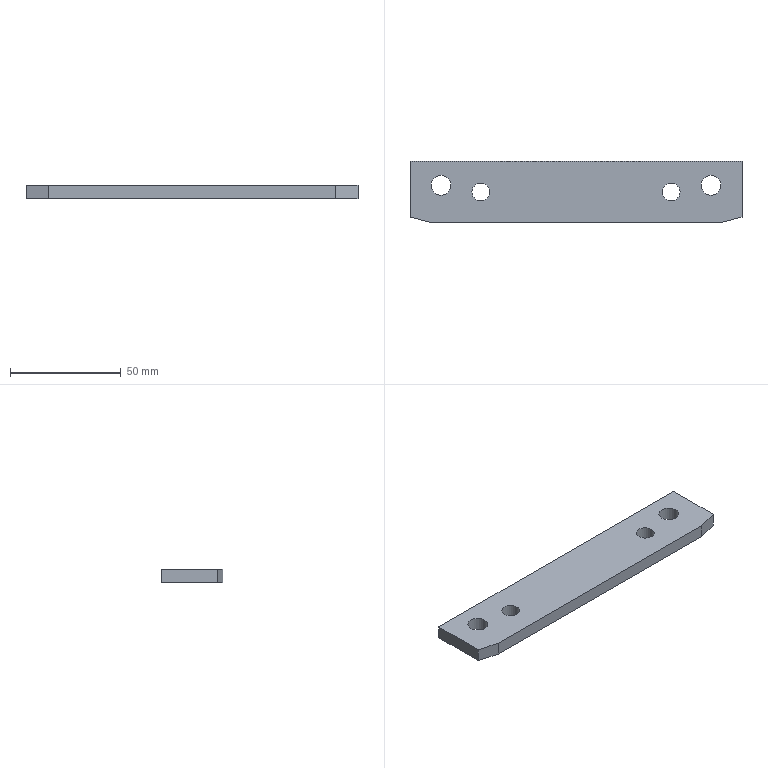Part | STEP file | gslz 2016.10.28-13_id1578_x_t | 1 solid | 12 faces | box 150 x 28 x 6 mm | volume 23673 mm3 | plane 8 | cylinder 4 | commonest cylinder face diameters 8 x2 9 x2
STEP:
#1=CARTESIAN_POINT('',(0.,0.,0.));
#2=DIRECTION('',(0.,0.,1.));
#3=DIRECTION('',(1.,0.,0.));
#4=AXIS2_PLACEMENT_3D('',#1,#2,#3);
#5=CARTESIAN_POINT('',(-1584.002,284.2,6.));
#6=VERTEX_POINT('',#5);
#7=CARTESIAN_POINT('',(-1592.002,284.2,6.));
#8=VERTEX_POINT('',#7);
#9=CARTESIAN_POINT('',(-1588.002,284.2,6.));
#10=DIRECTION('',(0.,0.,1.));
#11=DIRECTION('',(-1.,0.,0.));
#12=AXIS2_PLACEMENT_3D('',#9,#10,#11);
#13=CIRCLE('',#12,4.);
#14=CARTESIAN_POINT('',(-1588.002,284.2,-73.));
#15=DIRECTION('',(0.,0.,1.));
#16=DIRECTION('',(1.,0.,0.));
#17=AXIS2_PLACEMENT_3D('',#14,#15,#16);
#18=CYLINDRICAL_SURFACE('',#17,4.);
#19=CARTESIAN_POINT('',(-3.142,79.));
#20=DIRECTION('',(1.,0.));
#21=VECTOR('',#20,1.);
#22=LINE('',#19,#21);
#23=(GEOMETRIC_REPRESENTATION_CONTEXT(2)PARAMETRIC_REPRESENTATION_CONTEXT()REPRESENTATION_CONTEXT('',''));
#24=DEFINITIONAL_REPRESENTATION('',(#22),#23);
#25=PCURVE('',#18,#24);
#26=CARTESIAN_POINT('',(-1585.002,267.7,6.));
#27=DIRECTION('',(0.,0.,-1.));
#28=DIRECTION('',(-1.,0.,0.));
#29=AXIS2_PLACEMENT_3D('',#26,#27,#28);
#30=PLANE('',#29);
#31=CARTESIAN_POINT('',(7.,16.5));
#32=CARTESIAN_POINT('',(7.,9.572));
#33=CARTESIAN_POINT('',(1.,13.036));
#34=CARTESIAN_POINT('',(-5.,16.5));
#35=CARTESIAN_POINT('',(1.,19.964));
#36=CARTESIAN_POINT('',(7.,23.428));
#37=CARTESIAN_POINT('',(7.,16.5));
#38=(BOUNDED_CURVE()B_SPLINE_CURVE(2,(#31,#32,#33,#34,#35,#36,#37),.UNSPECIFIED.,.T.,.F.)B_SPLINE_CURVE_WITH_KNOTS((1,2,2,2,2,1),(-2.094,0.,2.094,4.189,6.283,8.378),.UNSPECIFIED.)CURVE()GEOMETRIC_REPRESENTATION_ITEM()RATIONAL_B_SPLINE_CURVE((1.,0.5,1.,0.5,1.,0.5,1.))REPRESENTATION_ITEM(''));
#39=(GEOMETRIC_REPRESENTATION_CONTEXT(2)PARAMETRIC_REPRESENTATION_CONTEXT()REPRESENTATION_CONTEXT('',''));
#40=DEFINITIONAL_REPRESENTATION('',(#38),#39);
#41=PCURVE('',#30,#40);
#42=SURFACE_CURVE('',#13,(#25,#41),.PCURVE_S1.);
#43=EDGE_CURVE('',#6,#8,#42,.T.);
#44=ORIENTED_EDGE('',*,*,#43,.F.);
#45=CARTESIAN_POINT('',(-1584.002,284.2,0.));
#46=VERTEX_POINT('',#45);
#47=CARTESIAN_POINT('',(-1584.002,284.2,0.));
#48=CARTESIAN_POINT('',(-1584.002,284.2,6.));
#49=B_SPLINE_CURVE_WITH_KNOTS('',1,(#47,#48),.UNSPECIFIED.,.F.,.F.,(2,2),(73.,79.),.PIECEWISE_BEZIER_KNOTS.);
#50=CARTESIAN_POINT('',(0.,0.));
#51=DIRECTION('',(0.,1.));
#52=VECTOR('',#51,1.);
#53=LINE('',#50,#52);
#54=(GEOMETRIC_REPRESENTATION_CONTEXT(2)PARAMETRIC_REPRESENTATION_CONTEXT()REPRESENTATION_CONTEXT('',''));
#55=DEFINITIONAL_REPRESENTATION('',(#53),#54);
#56=PCURVE('',#18,#55);
#57=CARTESIAN_POINT('',(6.283,0.));
#58=DIRECTION('',(0.,1.));
#59=VECTOR('',#58,1.);
#60=LINE('',#57,#59);
#61=(GEOMETRIC_REPRESENTATION_CONTEXT(2)PARAMETRIC_REPRESENTATION_CONTEXT()REPRESENTATION_CONTEXT('',''));
#62=DEFINITIONAL_REPRESENTATION('',(#60),#61);
#63=PCURVE('',#18,#62);
#64=SEAM_CURVE('',#49,(#56,#63),.PCURVE_S1.);
#65=EDGE_CURVE('',#46,#6,#64,.T.);
#66=ORIENTED_EDGE('',*,*,#65,.F.);
#67=CARTESIAN_POINT('',(-1588.002,284.2,0.));
#68=DIRECTION('',(0.,0.,-1.));
#69=DIRECTION('',(1.,0.,0.));
#70=AXIS2_PLACEMENT_3D('',#67,#68,#69);
#71=CIRCLE('',#70,4.);
#72=CARTESIAN_POINT('',(6.283,73.));
#73=DIRECTION('',(-1.,0.));
#74=VECTOR('',#73,1.);
#75=LINE('',#72,#74);
#76=(GEOMETRIC_REPRESENTATION_CONTEXT(2)PARAMETRIC_REPRESENTATION_CONTEXT()REPRESENTATION_CONTEXT('',''));
#77=DEFINITIONAL_REPRESENTATION('',(#75),#76);
#78=PCURVE('',#18,#77);
#79=CARTESIAN_POINT('',(-1625.002,298.2,0.));
#80=DIRECTION('',(0.,0.,1.));
#81=DIRECTION('',(1.,0.,0.));
#82=AXIS2_PLACEMENT_3D('',#79,#80,#81);
#83=PLANE('',#82);
#84=CARTESIAN_POINT('',(41.,-14.));
#85=CARTESIAN_POINT('',(41.,-20.928));
#86=CARTESIAN_POINT('',(35.,-17.464));
#87=CARTESIAN_POINT('',(29.,-14.));
#88=CARTESIAN_POINT('',(35.,-10.536));
#89=CARTESIAN_POINT('',(41.,-7.072));
#90=CARTESIAN_POINT('',(41.,-14.));
#91=(BOUNDED_CURVE()B_SPLINE_CURVE(2,(#84,#85,#86,#87,#88,#89,#90),.UNSPECIFIED.,.T.,.F.)B_SPLINE_CURVE_WITH_KNOTS((1,2,2,2,2,1),(-2.094,0.,2.094,4.189,6.283,8.378),.UNSPECIFIED.)CURVE()GEOMETRIC_REPRESENTATION_ITEM()RATIONAL_B_SPLINE_CURVE((1.,0.5,1.,0.5,1.,0.5,1.))REPRESENTATION_ITEM(''));
#92=(GEOMETRIC_REPRESENTATION_CONTEXT(2)PARAMETRIC_REPRESENTATION_CONTEXT()REPRESENTATION_CONTEXT('',''));
#93=DEFINITIONAL_REPRESENTATION('',(#91),#92);
#94=PCURVE('',#83,#93);
#95=SURFACE_CURVE('',#71,(#78,#94),.PCURVE_S1.);
#96=EDGE_CURVE('',#46,#46,#95,.T.);
#97=ORIENTED_EDGE('',*,*,#96,.F.);
#98=ORIENTED_EDGE('',*,*,#65,.T.);
#99=CARTESIAN_POINT('',(-1588.002,284.2,6.));
#100=DIRECTION('',(0.,0.,1.));
#101=DIRECTION('',(-1.,0.,0.));
#102=AXIS2_PLACEMENT_3D('',#99,#100,#101);
#103=CIRCLE('',#102,4.);
#104=CARTESIAN_POINT('',(3.142,79.));
#105=DIRECTION('',(1.,0.));
#106=VECTOR('',#105,1.);
#107=LINE('',#104,#106);
#108=(GEOMETRIC_REPRESENTATION_CONTEXT(2)PARAMETRIC_REPRESENTATION_CONTEXT()REPRESENTATION_CONTEXT('',''));
#109=DEFINITIONAL_REPRESENTATION('',(#107),#108);
#110=PCURVE('',#18,#109);
#111=CARTESIAN_POINT('',(7.,16.5));
#112=CARTESIAN_POINT('',(7.,9.572));
#113=CARTESIAN_POINT('',(1.,13.036));
#114=CARTESIAN_POINT('',(-5.,16.5));
#115=CARTESIAN_POINT('',(1.,19.964));
#116=CARTESIAN_POINT('',(7.,23.428));
#117=CARTESIAN_POINT('',(7.,16.5));
#118=(BOUNDED_CURVE()B_SPLINE_CURVE(2,(#111,#112,#113,#114,#115,#116,#117),.UNSPECIFIED.,.T.,.F.)B_SPLINE_CURVE_WITH_KNOTS((1,2,2,2,2,1),(-2.094,0.,2.094,4.189,6.283,8.378),.UNSPECIFIED.)CURVE()GEOMETRIC_REPRESENTATION_ITEM()RATIONAL_B_SPLINE_CURVE((1.,0.5,1.,0.5,1.,0.5,1.))REPRESENTATION_ITEM(''));
#119=(GEOMETRIC_REPRESENTATION_CONTEXT(2)PARAMETRIC_REPRESENTATION_CONTEXT()REPRESENTATION_CONTEXT('',''));
#120=DEFINITIONAL_REPRESENTATION('',(#118),#119);
#121=PCURVE('',#30,#120);
#122=SURFACE_CURVE('',#103,(#110,#121),.PCURVE_S1.);
#123=EDGE_CURVE('',#8,#6,#122,.T.);
#124=ORIENTED_EDGE('',*,*,#123,.F.);
#125=EDGE_LOOP('',(#44,#66,#97,#98,#124));
#126=FACE_BOUND('',#125,.F.);
#127=ADVANCED_FACE('',(#126),#18,.F.);
#128=CARTESIAN_POINT('',(-1506.002,284.2,6.));
#129=VERTEX_POINT('',#128);
#130=CARTESIAN_POINT('',(-1498.002,284.2,6.));
#131=VERTEX_POINT('',#130);
#132=CARTESIAN_POINT('',(-1502.002,284.2,6.));
#133=DIRECTION('',(0.,0.,-1.));
#134=DIRECTION('',(-1.,0.,0.));
#135=AXIS2_PLACEMENT_3D('',#132,#133,#134);
#136=CIRCLE('',#135,4.);
#137=CARTESIAN_POINT('',(-1502.002,284.2,-73.));
#138=DIRECTION('',(0.,0.,1.));
#139=DIRECTION('',(1.,0.,0.));
#140=AXIS2_PLACEMENT_3D('',#137,#138,#139);
#141=CYLINDRICAL_SURFACE('',#140,4.);
#142=CARTESIAN_POINT('',(3.142,79.));
#143=DIRECTION('',(-1.,0.));
#144=VECTOR('',#143,1.);
#145=LINE('',#142,#144);
#146=(GEOMETRIC_REPRESENTATION_CONTEXT(2)PARAMETRIC_REPRESENTATION_CONTEXT()REPRESENTATION_CONTEXT('',''));
#147=DEFINITIONAL_REPRESENTATION('',(#145),#146);
#148=PCURVE('',#141,#147);
#149=CARTESIAN_POINT('',(-83.,16.5));
#150=DIRECTION('',(1.,0.));
#151=AXIS2_PLACEMENT_2D('',#149,#150);
#152=CIRCLE('',#151,4.);
#153=(GEOMETRIC_REPRESENTATION_CONTEXT(2)PARAMETRIC_REPRESENTATION_CONTEXT()REPRESENTATION_CONTEXT('',''));
#154=DEFINITIONAL_REPRESENTATION('',(#152),#153);
#155=PCURVE('',#30,#154);
#156=SURFACE_CURVE('',#136,(#148,#155),.PCURVE_S1.);
#157=EDGE_CURVE('',#129,#131,#156,.T.);
#158=ORIENTED_EDGE('',*,*,#157,.T.);
#159=CARTESIAN_POINT('',(-1498.002,284.2,0.));
#160=VERTEX_POINT('',#159);
#161=CARTESIAN_POINT('',(-1498.002,284.2,0.));
#162=CARTESIAN_POINT('',(-1498.002,284.2,6.));
#163=B_SPLINE_CURVE_WITH_KNOTS('',1,(#161,#162),.UNSPECIFIED.,.F.,.F.,(2,2),(73.,79.),.PIECEWISE_BEZIER_KNOTS.);
#164=CARTESIAN_POINT('',(0.,0.));
#165=DIRECTION('',(0.,1.));
#166=VECTOR('',#165,1.);
#167=LINE('',#164,#166);
#168=(GEOMETRIC_REPRESENTATION_CONTEXT(2)PARAMETRIC_REPRESENTATION_CONTEXT()REPRESENTATION_CONTEXT('',''));
#169=DEFINITIONAL_REPRESENTATION('',(#167),#168);
#170=PCURVE('',#141,#169);
#171=CARTESIAN_POINT('',(6.283,0.));
#172=DIRECTION('',(0.,1.));
#173=VECTOR('',#172,1.);
#174=LINE('',#171,#173);
#175=(GEOMETRIC_REPRESENTATION_CONTEXT(2)PARAMETRIC_REPRESENTATION_CONTEXT()REPRESENTATION_CONTEXT('',''));
#176=DEFINITIONAL_REPRESENTATION('',(#174),#175);
#177=PCURVE('',#141,#176);
#178=SEAM_CURVE('',#163,(#170,#177),.PCURVE_S1.);
#179=EDGE_CURVE('',#160,#131,#178,.T.);
#180=ORIENTED_EDGE('',*,*,#179,.F.);
#181=CARTESIAN_POINT('',(-1502.002,284.2,0.));
#182=DIRECTION('',(0.,0.,1.));
#183=DIRECTION('',(1.,0.,0.));
#184=AXIS2_PLACEMENT_3D('',#181,#182,#183);
#185=CIRCLE('',#184,4.);
#186=CARTESIAN_POINT('',(0.,73.));
#187=DIRECTION('',(1.,0.));
#188=VECTOR('',#187,1.);
#189=LINE('',#186,#188);
#190=(GEOMETRIC_REPRESENTATION_CONTEXT(2)PARAMETRIC_REPRESENTATION_CONTEXT()REPRESENTATION_CONTEXT('',''));
#191=DEFINITIONAL_REPRESENTATION('',(#189),#190);
#192=PCURVE('',#141,#191);
#193=CARTESIAN_POINT('',(123.,-14.));
#194=DIRECTION('',(1.,0.));
#195=AXIS2_PLACEMENT_2D('',#193,#194);
#196=CIRCLE('',#195,4.);
#197=(GEOMETRIC_REPRESENTATION_CONTEXT(2)PARAMETRIC_REPRESENTATION_CONTEXT()REPRESENTATION_CONTEXT('',''));
#198=DEFINITIONAL_REPRESENTATION('',(#196),#197);
#199=PCURVE('',#83,#198);
#200=SURFACE_CURVE('',#185,(#192,#199),.PCURVE_S1.);
#201=EDGE_CURVE('',#160,#160,#200,.T.);
#202=ORIENTED_EDGE('',*,*,#201,.T.);
#203=ORIENTED_EDGE('',*,*,#179,.T.);
#204=CARTESIAN_POINT('',(-1502.002,284.2,6.));
#205=DIRECTION('',(0.,0.,-1.));
#206=DIRECTION('',(-1.,0.,0.));
#207=AXIS2_PLACEMENT_3D('',#204,#205,#206);
#208=CIRCLE('',#207,4.);
#209=CARTESIAN_POINT('',(9.425,79.));
#210=DIRECTION('',(-1.,0.));
#211=VECTOR('',#210,1.);
#212=LINE('',#209,#211);
#213=(GEOMETRIC_REPRESENTATION_CONTEXT(2)PARAMETRIC_REPRESENTATION_CONTEXT()REPRESENTATION_CONTEXT('',''));
#214=DEFINITIONAL_REPRESENTATION('',(#212),#213);
#215=PCURVE('',#141,#214);
#216=CARTESIAN_POINT('',(-83.,16.5));
#217=DIRECTION('',(1.,0.));
#218=AXIS2_PLACEMENT_2D('',#216,#217);
#219=CIRCLE('',#218,4.);
#220=(GEOMETRIC_REPRESENTATION_CONTEXT(2)PARAMETRIC_REPRESENTATION_CONTEXT()REPRESENTATION_CONTEXT('',''));
#221=DEFINITIONAL_REPRESENTATION('',(#219),#220);
#222=PCURVE('',#30,#221);
#223=SURFACE_CURVE('',#208,(#215,#222),.PCURVE_S1.);
#224=EDGE_CURVE('',#131,#129,#223,.T.);
#225=ORIENTED_EDGE('',*,*,#224,.T.);
#226=EDGE_LOOP('',(#158,#180,#202,#203,#225));
#227=FACE_BOUND('',#226,.F.);
#228=ADVANCED_FACE('',(#227),#141,.F.);
#229=CARTESIAN_POINT('',(-1610.502,287.2,6.));
#230=VERTEX_POINT('',#229);
#231=CARTESIAN_POINT('',(-1606.002,287.2,6.));
#232=DIRECTION('',(0.,0.,-1.));
#233=DIRECTION('',(-1.,0.,0.));
#234=AXIS2_PLACEMENT_3D('',#231,#232,#233);
#235=CIRCLE('',#234,4.5);
#236=CARTESIAN_POINT('',(-1606.002,287.2,47.));
#237=DIRECTION('',(0.,0.,-1.));
#238=DIRECTION('',(-1.,0.,0.));
#239=AXIS2_PLACEMENT_3D('',#236,#237,#238);
#240=CYLINDRICAL_SURFACE('',#239,4.5);
#241=CARTESIAN_POINT('',(0.,41.));
#242=DIRECTION('',(1.,0.));
#243=VECTOR('',#242,1.);
#244=LINE('',#241,#243);
#245=(GEOMETRIC_REPRESENTATION_CONTEXT(2)PARAMETRIC_REPRESENTATION_CONTEXT()REPRESENTATION_CONTEXT('',''));
#246=DEFINITIONAL_REPRESENTATION('',(#244),#245);
#247=PCURVE('',#240,#246);
#248=CARTESIAN_POINT('',(21.,19.5));
#249=DIRECTION('',(1.,0.));
#250=AXIS2_PLACEMENT_2D('',#248,#249);
#251=CIRCLE('',#250,4.5);
#252=(GEOMETRIC_REPRESENTATION_CONTEXT(2)PARAMETRIC_REPRESENTATION_CONTEXT()REPRESENTATION_CONTEXT('',''));
#253=DEFINITIONAL_REPRESENTATION('',(#251),#252);
#254=PCURVE('',#30,#253);
#255=SURFACE_CURVE('',#235,(#247,#254),.PCURVE_S1.);
#256=EDGE_CURVE('',#230,#230,#255,.T.);
#257=ORIENTED_EDGE('',*,*,#256,.T.);
#258=CARTESIAN_POINT('',(-1610.502,287.2,0.));
#259=VERTEX_POINT('',#258);
#260=CARTESIAN_POINT('',(-1610.502,287.2,6.));
#261=CARTESIAN_POINT('',(-1610.502,287.2,0.));
#262=B_SPLINE_CURVE_WITH_KNOTS('',1,(#260,#261),.UNSPECIFIED.,.F.,.F.,(2,2),(41.,47.),.PIECEWISE_BEZIER_KNOTS.);
#263=CARTESIAN_POINT('',(6.283,0.));
#264=DIRECTION('',(0.,1.));
#265=VECTOR('',#264,1.);
#266=LINE('',#263,#265);
#267=(GEOMETRIC_REPRESENTATION_CONTEXT(2)PARAMETRIC_REPRESENTATION_CONTEXT()REPRESENTATION_CONTEXT('',''));
#268=DEFINITIONAL_REPRESENTATION('',(#266),#267);
#269=PCURVE('',#240,#268);
#270=CARTESIAN_POINT('',(0.,0.));
#271=DIRECTION('',(0.,1.));
#272=VECTOR('',#271,1.);
#273=LINE('',#270,#272);
#274=(GEOMETRIC_REPRESENTATION_CONTEXT(2)PARAMETRIC_REPRESENTATION_CONTEXT()REPRESENTATION_CONTEXT('',''));
#275=DEFINITIONAL_REPRESENTATION('',(#273),#274);
#276=PCURVE('',#240,#275);
#277=SEAM_CURVE('',#262,(#269,#276),.PCURVE_S1.);
#278=EDGE_CURVE('',#230,#259,#277,.T.);
#279=ORIENTED_EDGE('',*,*,#278,.T.);
#280=CARTESIAN_POINT('',(-1601.502,287.2,0.));
#281=VERTEX_POINT('',#280);
#282=CARTESIAN_POINT('',(-1606.002,287.2,0.));
#283=DIRECTION('',(0.,0.,1.));
#284=DIRECTION('',(1.,0.,0.));
#285=AXIS2_PLACEMENT_3D('',#282,#283,#284);
#286=CIRCLE('',#285,4.5);
#287=CARTESIAN_POINT('',(9.425,47.));
#288=DIRECTION('',(-1.,0.));
#289=VECTOR('',#288,1.);
#290=LINE('',#287,#289);
#291=(GEOMETRIC_REPRESENTATION_CONTEXT(2)PARAMETRIC_REPRESENTATION_CONTEXT()REPRESENTATION_CONTEXT('',''));
#292=DEFINITIONAL_REPRESENTATION('',(#290),#291);
#293=PCURVE('',#240,#292);
#294=CARTESIAN_POINT('',(19.,-11.));
#295=DIRECTION('',(1.,0.));
#296=AXIS2_PLACEMENT_2D('',#294,#295);
#297=CIRCLE('',#296,4.5);
#298=(GEOMETRIC_REPRESENTATION_CONTEXT(2)PARAMETRIC_REPRESENTATION_CONTEXT()REPRESENTATION_CONTEXT('',''));
#299=DEFINITIONAL_REPRESENTATION('',(#297),#298);
#300=PCURVE('',#83,#299);
#301=SURFACE_CURVE('',#286,(#293,#300),.PCURVE_S1.);
#302=EDGE_CURVE('',#259,#281,#301,.T.);
#303=ORIENTED_EDGE('',*,*,#302,.T.);
#304=CARTESIAN_POINT('',(-1606.002,287.2,0.));
#305=DIRECTION('',(0.,0.,1.));
#306=DIRECTION('',(1.,0.,0.));
#307=AXIS2_PLACEMENT_3D('',#304,#305,#306);
#308=CIRCLE('',#307,4.5);
#309=CARTESIAN_POINT('',(3.142,47.));
#310=DIRECTION('',(-1.,0.));
#311=VECTOR('',#310,1.);
#312=LINE('',#309,#311);
#313=(GEOMETRIC_REPRESENTATION_CONTEXT(2)PARAMETRIC_REPRESENTATION_CONTEXT()REPRESENTATION_CONTEXT('',''));
#314=DEFINITIONAL_REPRESENTATION('',(#312),#313);
#315=PCURVE('',#240,#314);
#316=CARTESIAN_POINT('',(19.,-11.));
#317=DIRECTION('',(1.,0.));
#318=AXIS2_PLACEMENT_2D('',#316,#317);
#319=CIRCLE('',#318,4.5);
#320=(GEOMETRIC_REPRESENTATION_CONTEXT(2)PARAMETRIC_REPRESENTATION_CONTEXT()REPRESENTATION_CONTEXT('',''));
#321=DEFINITIONAL_REPRESENTATION('',(#319),#320);
#322=PCURVE('',#83,#321);
#323=SURFACE_CURVE('',#308,(#315,#322),.PCURVE_S1.);
#324=EDGE_CURVE('',#281,#259,#323,.T.);
#325=ORIENTED_EDGE('',*,*,#324,.T.);
#326=ORIENTED_EDGE('',*,*,#278,.F.);
#327=EDGE_LOOP('',(#257,#279,#303,#325,#326));
#328=FACE_BOUND('',#327,.F.);
#329=ADVANCED_FACE('',(#328),#240,.F.);
#330=CARTESIAN_POINT('',(-1480.001,270.2,0.));
#331=VERTEX_POINT('',#330);
#332=CARTESIAN_POINT('',(-1480.001,270.2,6.));
#333=VERTEX_POINT('',#332);
#334=CARTESIAN_POINT('',(-1480.001,270.2,8.));
#335=DIRECTION('',(0.,0.,1.));
#336=VECTOR('',#335,1.);
#337=LINE('',#334,#336);
#338=CARTESIAN_POINT('',(-1615.,270.2,8.));
#339=DIRECTION('',(0.,1.,0.));
#340=DIRECTION('',(0.,0.,1.));
#341=AXIS2_PLACEMENT_3D('',#338,#339,#340);
#342=PLANE('',#341);
#343=CARTESIAN_POINT('',(0.,134.999));
#344=DIRECTION('',(1.,0.));
#345=VECTOR('',#344,1.);
#346=LINE('',#343,#345);
#347=(GEOMETRIC_REPRESENTATION_CONTEXT(2)PARAMETRIC_REPRESENTATION_CONTEXT()REPRESENTATION_CONTEXT('',''));
#348=DEFINITIONAL_REPRESENTATION('',(#346),#347);
#349=PCURVE('',#342,#348);
#350=CARTESIAN_POINT('',(-1480.001,270.2,8.));
#351=DIRECTION('',(-0.2588,0.9659,0.));
#352=DIRECTION('',(-0.9659,-0.2588,0.));
#353=AXIS2_PLACEMENT_3D('',#350,#351,#352);
#354=PLANE('',#353);
#355=CARTESIAN_POINT('',(0.,0.));
#356=DIRECTION('',(0.,1.));
#357=VECTOR('',#356,1.);
#358=LINE('',#355,#357);
#359=(GEOMETRIC_REPRESENTATION_CONTEXT(2)PARAMETRIC_REPRESENTATION_CONTEXT()REPRESENTATION_CONTEXT('',''));
#360=DEFINITIONAL_REPRESENTATION('',(#358),#359);
#361=PCURVE('',#354,#360);
#362=SURFACE_CURVE('',#337,(#349,#361),.PCURVE_S1.);
#363=EDGE_CURVE('',#331,#333,#362,.T.);
#364=ORIENTED_EDGE('',*,*,#363,.T.);
#365=CARTESIAN_POINT('',(-1610.,270.2,6.));
#366=VERTEX_POINT('',#365);
#367=CARTESIAN_POINT('',(-1615.,270.2,6.));
#368=DIRECTION('',(-1.,0.,0.));
#369=VECTOR('',#368,1.);
#370=LINE('',#367,#369);
#371=CARTESIAN_POINT('',(-2.,0.));
#372=DIRECTION('',(0.,-1.));
#373=VECTOR('',#372,1.);
#374=LINE('',#371,#373);
#375=(GEOMETRIC_REPRESENTATION_CONTEXT(2)PARAMETRIC_REPRESENTATION_CONTEXT()REPRESENTATION_CONTEXT('',''));
#376=DEFINITIONAL_REPRESENTATION('',(#374),#375);
#377=PCURVE('',#342,#376);
#378=CARTESIAN_POINT('',(29.998,2.5));
#379=DIRECTION('',(1.,0.));
#380=VECTOR('',#379,1.);
#381=LINE('',#378,#380);
#382=(GEOMETRIC_REPRESENTATION_CONTEXT(2)PARAMETRIC_REPRESENTATION_CONTEXT()REPRESENTATION_CONTEXT('',''));
#383=DEFINITIONAL_REPRESENTATION('',(#381),#382);
#384=PCURVE('',#30,#383);
#385=SURFACE_CURVE('',#370,(#377,#384),.PCURVE_S1.);
#386=EDGE_CURVE('',#333,#366,#385,.T.);
#387=ORIENTED_EDGE('',*,*,#386,.T.);
#388=CARTESIAN_POINT('',(-1610.,270.2,0.));
#389=VERTEX_POINT('',#388);
#390=CARTESIAN_POINT('',(-1610.,270.2,8.));
#391=DIRECTION('',(0.,0.,1.));
#392=VECTOR('',#391,1.);
#393=LINE('',#390,#392);
#394=CARTESIAN_POINT('',(0.,5.));
#395=DIRECTION('',(1.,0.));
#396=VECTOR('',#395,1.);
#397=LINE('',#394,#396);
#398=(GEOMETRIC_REPRESENTATION_CONTEXT(2)PARAMETRIC_REPRESENTATION_CONTEXT()REPRESENTATION_CONTEXT('',''));
#399=DEFINITIONAL_REPRESENTATION('',(#397),#398);
#400=PCURVE('',#342,#399);
#401=CARTESIAN_POINT('',(-1620.002,272.88,8.));
#402=DIRECTION('',(0.2588,0.9659,0.));
#403=DIRECTION('',(-0.9659,0.2588,0.));
#404=AXIS2_PLACEMENT_3D('',#401,#402,#403);
#405=PLANE('',#404);
#406=CARTESIAN_POINT('',(-10.355,0.));
#407=DIRECTION('',(0.,1.));
#408=VECTOR('',#407,1.);
#409=LINE('',#406,#408);
#410=(GEOMETRIC_REPRESENTATION_CONTEXT(2)PARAMETRIC_REPRESENTATION_CONTEXT()REPRESENTATION_CONTEXT('',''));
#411=DEFINITIONAL_REPRESENTATION('',(#409),#410);
#412=PCURVE('',#405,#411);
#413=SURFACE_CURVE('',#393,(#400,#412),.PCURVE_S1.);
#414=EDGE_CURVE('',#389,#366,#413,.T.);
#415=ORIENTED_EDGE('',*,*,#414,.F.);
#416=CARTESIAN_POINT('',(-1615.,270.2,0.));
#417=DIRECTION('',(1.,0.,0.));
#418=VECTOR('',#417,1.);
#419=LINE('',#416,#418);
#420=CARTESIAN_POINT('',(-8.,0.));
#421=DIRECTION('',(0.,1.));
#422=VECTOR('',#421,1.);
#423=LINE('',#420,#422);
#424=(GEOMETRIC_REPRESENTATION_CONTEXT(2)PARAMETRIC_REPRESENTATION_CONTEXT()REPRESENTATION_CONTEXT('',''));
#425=DEFINITIONAL_REPRESENTATION('',(#423),#424);
#426=PCURVE('',#342,#425);
#427=CARTESIAN_POINT('',(10.002,-28.));
#428=DIRECTION('',(1.,0.));
#429=VECTOR('',#428,1.);
#430=LINE('',#427,#429);
#431=(GEOMETRIC_REPRESENTATION_CONTEXT(2)PARAMETRIC_REPRESENTATION_CONTEXT()REPRESENTATION_CONTEXT('',''));
#432=DEFINITIONAL_REPRESENTATION('',(#430),#431);
#433=PCURVE('',#83,#432);
#434=SURFACE_CURVE('',#419,(#426,#433),.PCURVE_S1.);
#435=EDGE_CURVE('',#389,#331,#434,.T.);
#436=ORIENTED_EDGE('',*,*,#435,.T.);
#437=EDGE_LOOP('',(#364,#387,#415,#436));
#438=FACE_BOUND('',#437,.T.);
#439=ADVANCED_FACE('',(#438),#342,.F.);
#440=CARTESIAN_POINT('',(-1470.002,272.879,6.));
#441=VERTEX_POINT('',#440);
#442=CARTESIAN_POINT('',(-1470.002,272.879,0.));
#443=VERTEX_POINT('',#442);
#444=CARTESIAN_POINT('',(-1470.002,272.879,8.));
#445=DIRECTION('',(0.,0.,-1.));
#446=VECTOR('',#445,1.);
#447=LINE('',#444,#446);
#448=CARTESIAN_POINT('',(-10.352,0.));
#449=DIRECTION('',(0.,-1.));
#450=VECTOR('',#449,1.);
#451=LINE('',#448,#450);
#452=(GEOMETRIC_REPRESENTATION_CONTEXT(2)PARAMETRIC_REPRESENTATION_CONTEXT()REPRESENTATION_CONTEXT('',''));
#453=DEFINITIONAL_REPRESENTATION('',(#451),#452);
#454=PCURVE('',#354,#453);
#455=CARTESIAN_POINT('',(-1470.002,265.2,16.));
#456=DIRECTION('',(-1.,0.,0.));
#457=DIRECTION('',(0.,0.,1.));
#458=AXIS2_PLACEMENT_3D('',#455,#456,#457);
#459=PLANE('',#458);
#460=CARTESIAN_POINT('',(-8.,7.679));
#461=DIRECTION('',(-1.,0.));
#462=VECTOR('',#461,1.);
#463=LINE('',#460,#462);
#464=(GEOMETRIC_REPRESENTATION_CONTEXT(2)PARAMETRIC_REPRESENTATION_CONTEXT()REPRESENTATION_CONTEXT('',''));
#465=DEFINITIONAL_REPRESENTATION('',(#463),#464);
#466=PCURVE('',#459,#465);
#467=SURFACE_CURVE('',#447,(#454,#466),.PCURVE_S1.);
#468=EDGE_CURVE('',#441,#443,#467,.T.);
#469=ORIENTED_EDGE('',*,*,#468,.F.);
#470=CARTESIAN_POINT('',(-1480.001,270.2,6.));
#471=DIRECTION('',(-0.9659,-0.2588,0.));
#472=VECTOR('',#471,1.);
#473=LINE('',#470,#472);
#474=CARTESIAN_POINT('',(0.,-2.));
#475=DIRECTION('',(1.,0.));
#476=VECTOR('',#475,1.);
#477=LINE('',#474,#476);
#478=(GEOMETRIC_REPRESENTATION_CONTEXT(2)PARAMETRIC_REPRESENTATION_CONTEXT()REPRESENTATION_CONTEXT('',''));
#479=DEFINITIONAL_REPRESENTATION('',(#477),#478);
#480=PCURVE('',#354,#479);
#481=CARTESIAN_POINT('',(-105.001,2.5));
#482=DIRECTION('',(0.9659,-0.2588));
#483=VECTOR('',#482,1.);
#484=LINE('',#481,#483);
#485=(GEOMETRIC_REPRESENTATION_CONTEXT(2)PARAMETRIC_REPRESENTATION_CONTEXT()REPRESENTATION_CONTEXT('',''));
#486=DEFINITIONAL_REPRESENTATION('',(#484),#485);
#487=PCURVE('',#30,#486);
#488=SURFACE_CURVE('',#473,(#480,#487),.PCURVE_S1.);
#489=EDGE_CURVE('',#441,#333,#488,.T.);
#490=ORIENTED_EDGE('',*,*,#489,.T.);
#491=ORIENTED_EDGE('',*,*,#363,.F.);
#492=CARTESIAN_POINT('',(-1480.001,270.2,0.));
#493=DIRECTION('',(0.9659,0.2588,0.));
#494=VECTOR('',#493,1.);
#495=LINE('',#492,#494);
#496=CARTESIAN_POINT('',(0.,-8.));
#497=DIRECTION('',(-1.,0.));
#498=VECTOR('',#497,1.);
#499=LINE('',#496,#498);
#500=(GEOMETRIC_REPRESENTATION_CONTEXT(2)PARAMETRIC_REPRESENTATION_CONTEXT()REPRESENTATION_CONTEXT('',''));
#501=DEFINITIONAL_REPRESENTATION('',(#499),#500);
#502=PCURVE('',#354,#501);
#503=CARTESIAN_POINT('',(145.001,-28.));
#504=DIRECTION('',(0.9659,0.2588));
#505=VECTOR('',#504,1.);
#506=LINE('',#503,#505);
#507=(GEOMETRIC_REPRESENTATION_CONTEXT(2)PARAMETRIC_REPRESENTATION_CONTEXT()REPRESENTATION_CONTEXT('',''));
#508=DEFINITIONAL_REPRESENTATION('',(#506),#507);
#509=PCURVE('',#83,#508);
#510=SURFACE_CURVE('',#495,(#502,#509),.PCURVE_S1.);
#511=EDGE_CURVE('',#331,#443,#510,.T.);
#512=ORIENTED_EDGE('',*,*,#511,.T.);
#513=EDGE_LOOP('',(#469,#490,#491,#512));
#514=FACE_BOUND('',#513,.T.);
#515=ADVANCED_FACE('',(#514),#354,.F.);
#516=CARTESIAN_POINT('',(-1470.002,298.2,6.));
#517=VERTEX_POINT('',#516);
#518=CARTESIAN_POINT('',(-1470.002,298.2,0.));
#519=VERTEX_POINT('',#518);
#520=CARTESIAN_POINT('',(-1470.002,298.2,16.));
#521=DIRECTION('',(0.,0.,-1.));
#522=VECTOR('',#521,1.);
#523=LINE('',#520,#522);
#524=CARTESIAN_POINT('',(0.,33.));
#525=DIRECTION('',(-1.,0.));
#526=VECTOR('',#525,1.);
#527=LINE('',#524,#526);
#528=(GEOMETRIC_REPRESENTATION_CONTEXT(2)PARAMETRIC_REPRESENTATION_CONTEXT()REPRESENTATION_CONTEXT('',''));
#529=DEFINITIONAL_REPRESENTATION('',(#527),#528);
#530=PCURVE('',#459,#529);
#531=CARTESIAN_POINT('',(-1545.002,298.2,16.));
#532=DIRECTION('',(0.,-1.,0.));
#533=DIRECTION('',(0.,0.,-1.));
#534=AXIS2_PLACEMENT_3D('',#531,#532,#533);
#535=PLANE('',#534);
#536=CARTESIAN_POINT('',(0.,75.));
#537=DIRECTION('',(1.,0.));
#538=VECTOR('',#537,1.);
#539=LINE('',#536,#538);
#540=(GEOMETRIC_REPRESENTATION_CONTEXT(2)PARAMETRIC_REPRESENTATION_CONTEXT()REPRESENTATION_CONTEXT('',''));
#541=DEFINITIONAL_REPRESENTATION('',(#539),#540);
#542=PCURVE('',#535,#541);
#543=SURFACE_CURVE('',#523,(#530,#542),.PCURVE_S1.);
#544=EDGE_CURVE('',#517,#519,#543,.T.);
#545=ORIENTED_EDGE('',*,*,#544,.F.);
#546=CARTESIAN_POINT('',(-1470.002,265.2,6.));
#547=DIRECTION('',(0.,-1.,0.));
#548=VECTOR('',#547,1.);
#549=LINE('',#546,#548);
#550=CARTESIAN_POINT('',(-10.,0.));
#551=DIRECTION('',(0.,-1.));
#552=VECTOR('',#551,1.);
#553=LINE('',#550,#552);
#554=(GEOMETRIC_REPRESENTATION_CONTEXT(2)PARAMETRIC_REPRESENTATION_CONTEXT()REPRESENTATION_CONTEXT('',''));
#555=DEFINITIONAL_REPRESENTATION('',(#553),#554);
#556=PCURVE('',#459,#555);
#557=CARTESIAN_POINT('',(-115.,-2.5));
#558=DIRECTION('',(0.,-1.));
#559=VECTOR('',#558,1.);
#560=LINE('',#557,#559);
#561=(GEOMETRIC_REPRESENTATION_CONTEXT(2)PARAMETRIC_REPRESENTATION_CONTEXT()REPRESENTATION_CONTEXT('',''));
#562=DEFINITIONAL_REPRESENTATION('',(#560),#561);
#563=PCURVE('',#30,#562);
#564=SURFACE_CURVE('',#549,(#556,#563),.PCURVE_S1.);
#565=EDGE_CURVE('',#517,#441,#564,.T.);
#566=ORIENTED_EDGE('',*,*,#565,.T.);
#567=ORIENTED_EDGE('',*,*,#468,.T.);
#568=CARTESIAN_POINT('',(-1470.002,265.2,0.));
#569=DIRECTION('',(0.,1.,0.));
#570=VECTOR('',#569,1.);
#571=LINE('',#568,#570);
#572=CARTESIAN_POINT('',(-16.,0.));
#573=DIRECTION('',(0.,1.));
#574=VECTOR('',#573,1.);
#575=LINE('',#572,#574);
#576=(GEOMETRIC_REPRESENTATION_CONTEXT(2)PARAMETRIC_REPRESENTATION_CONTEXT()REPRESENTATION_CONTEXT('',''));
#577=DEFINITIONAL_REPRESENTATION('',(#575),#576);
#578=PCURVE('',#459,#577);
#579=CARTESIAN_POINT('',(155.,-33.));
#580=DIRECTION('',(0.,1.));
#581=VECTOR('',#580,1.);
#582=LINE('',#579,#581);
#583=(GEOMETRIC_REPRESENTATION_CONTEXT(2)PARAMETRIC_REPRESENTATION_CONTEXT()REPRESENTATION_CONTEXT('',''));
#584=DEFINITIONAL_REPRESENTATION('',(#582),#583);
#585=PCURVE('',#83,#584);
#586=SURFACE_CURVE('',#571,(#578,#585),.PCURVE_S1.);
#587=EDGE_CURVE('',#443,#519,#586,.T.);
#588=ORIENTED_EDGE('',*,*,#587,.T.);
#589=EDGE_LOOP('',(#545,#566,#567,#588));
#590=FACE_BOUND('',#589,.T.);
#591=ADVANCED_FACE('',(#590),#459,.F.);
#592=CARTESIAN_POINT('',(-1620.002,298.2,6.));
#593=VERTEX_POINT('',#592);
#594=CARTESIAN_POINT('',(-1620.002,298.2,0.));
#595=VERTEX_POINT('',#594);
#596=CARTESIAN_POINT('',(-1620.002,298.2,16.));
#597=DIRECTION('',(0.,0.,-1.));
#598=VECTOR('',#597,1.);
#599=LINE('',#596,#598);
#600=CARTESIAN_POINT('',(0.,-75.));
#601=DIRECTION('',(1.,0.));
#602=VECTOR('',#601,1.);
#603=LINE('',#600,#602);
#604=(GEOMETRIC_REPRESENTATION_CONTEXT(2)PARAMETRIC_REPRESENTATION_CONTEXT()REPRESENTATION_CONTEXT('',''));
#605=DEFINITIONAL_REPRESENTATION('',(#603),#604);
#606=PCURVE('',#535,#605);
#607=CARTESIAN_POINT('',(-1620.002,298.2,16.));
#608=DIRECTION('',(1.,0.,0.));
#609=DIRECTION('',(0.,0.,-1.));
#610=AXIS2_PLACEMENT_3D('',#607,#608,#609);
#611=PLANE('',#610);
#612=CARTESIAN_POINT('',(0.,0.));
#613=DIRECTION('',(1.,0.));
#614=VECTOR('',#613,1.);
#615=LINE('',#612,#614);
#616=(GEOMETRIC_REPRESENTATION_CONTEXT(2)PARAMETRIC_REPRESENTATION_CONTEXT()REPRESENTATION_CONTEXT('',''));
#617=DEFINITIONAL_REPRESENTATION('',(#615),#616);
#618=PCURVE('',#611,#617);
#619=SURFACE_CURVE('',#599,(#606,#618),.PCURVE_S1.);
#620=EDGE_CURVE('',#593,#595,#619,.T.);
#621=ORIENTED_EDGE('',*,*,#620,.F.);
#622=CARTESIAN_POINT('',(-1545.002,298.2,6.));
#623=DIRECTION('',(1.,0.,0.));
#624=VECTOR('',#623,1.);
#625=LINE('',#622,#624);
#626=CARTESIAN_POINT('',(10.,0.));
#627=DIRECTION('',(0.,1.));
#628=VECTOR('',#627,1.);
#629=LINE('',#626,#628);
#630=(GEOMETRIC_REPRESENTATION_CONTEXT(2)PARAMETRIC_REPRESENTATION_CONTEXT()REPRESENTATION_CONTEXT('',''));
#631=DEFINITIONAL_REPRESENTATION('',(#629),#630);
#632=PCURVE('',#535,#631);
#633=CARTESIAN_POINT('',(-40.,30.5));
#634=DIRECTION('',(-1.,0.));
#635=VECTOR('',#634,1.);
#636=LINE('',#633,#635);
#637=(GEOMETRIC_REPRESENTATION_CONTEXT(2)PARAMETRIC_REPRESENTATION_CONTEXT()REPRESENTATION_CONTEXT('',''));
#638=DEFINITIONAL_REPRESENTATION('',(#636),#637);
#639=PCURVE('',#30,#638);
#640=SURFACE_CURVE('',#625,(#632,#639),.PCURVE_S1.);
#641=EDGE_CURVE('',#593,#517,#640,.T.);
#642=ORIENTED_EDGE('',*,*,#641,.T.);
#643=ORIENTED_EDGE('',*,*,#544,.T.);
#644=CARTESIAN_POINT('',(-1545.002,298.2,0.));
#645=DIRECTION('',(-1.,0.,0.));
#646=VECTOR('',#645,1.);
#647=LINE('',#644,#646);
#648=CARTESIAN_POINT('',(16.,0.));
#649=DIRECTION('',(0.,-1.));
#650=VECTOR('',#649,1.);
#651=LINE('',#648,#650);
#652=(GEOMETRIC_REPRESENTATION_CONTEXT(2)PARAMETRIC_REPRESENTATION_CONTEXT()REPRESENTATION_CONTEXT('',''));
#653=DEFINITIONAL_REPRESENTATION('',(#651),#652);
#654=PCURVE('',#535,#653);
#655=CARTESIAN_POINT('',(80.,0.));
#656=DIRECTION('',(-1.,0.));
#657=VECTOR('',#656,1.);
#658=LINE('',#655,#657);
#659=(GEOMETRIC_REPRESENTATION_CONTEXT(2)PARAMETRIC_REPRESENTATION_CONTEXT()REPRESENTATION_CONTEXT('',''));
#660=DEFINITIONAL_REPRESENTATION('',(#658),#659);
#661=PCURVE('',#83,#660);
#662=SURFACE_CURVE('',#647,(#654,#661),.PCURVE_S1.);
#663=EDGE_CURVE('',#519,#595,#662,.T.);
#664=ORIENTED_EDGE('',*,*,#663,.T.);
#665=EDGE_LOOP('',(#621,#642,#643,#664));
#666=FACE_BOUND('',#665,.T.);
#667=ADVANCED_FACE('',(#666),#535,.F.);
#668=CARTESIAN_POINT('',(-1620.002,272.88,6.));
#669=VERTEX_POINT('',#668);
#670=CARTESIAN_POINT('',(-1620.002,272.88,0.));
#671=VERTEX_POINT('',#670);
#672=CARTESIAN_POINT('',(-1620.002,272.88,8.));
#673=DIRECTION('',(0.,0.,-1.));
#674=VECTOR('',#673,1.);
#675=LINE('',#672,#674);
#676=CARTESIAN_POINT('',(8.,-25.32));
#677=DIRECTION('',(1.,0.));
#678=VECTOR('',#677,1.);
#679=LINE('',#676,#678);
#680=(GEOMETRIC_REPRESENTATION_CONTEXT(2)PARAMETRIC_REPRESENTATION_CONTEXT()REPRESENTATION_CONTEXT('',''));
#681=DEFINITIONAL_REPRESENTATION('',(#679),#680);
#682=PCURVE('',#611,#681);
#683=CARTESIAN_POINT('',(0.,0.));
#684=DIRECTION('',(0.,-1.));
#685=VECTOR('',#684,1.);
#686=LINE('',#683,#685);
#687=(GEOMETRIC_REPRESENTATION_CONTEXT(2)PARAMETRIC_REPRESENTATION_CONTEXT()REPRESENTATION_CONTEXT('',''));
#688=DEFINITIONAL_REPRESENTATION('',(#686),#687);
#689=PCURVE('',#405,#688);
#690=SURFACE_CURVE('',#675,(#682,#689),.PCURVE_S1.);
#691=EDGE_CURVE('',#669,#671,#690,.T.);
#692=ORIENTED_EDGE('',*,*,#691,.F.);
#693=CARTESIAN_POINT('',(-1620.002,298.2,6.));
#694=DIRECTION('',(0.,1.,0.));
#695=VECTOR('',#694,1.);
#696=LINE('',#693,#695);
#697=CARTESIAN_POINT('',(10.,0.));
#698=DIRECTION('',(0.,1.));
#699=VECTOR('',#698,1.);
#700=LINE('',#697,#699);
#701=(GEOMETRIC_REPRESENTATION_CONTEXT(2)PARAMETRIC_REPRESENTATION_CONTEXT()REPRESENTATION_CONTEXT('',''));
#702=DEFINITIONAL_REPRESENTATION('',(#700),#701);
#703=PCURVE('',#611,#702);
#704=CARTESIAN_POINT('',(35.,30.5));
#705=DIRECTION('',(0.,1.));
#706=VECTOR('',#705,1.);
#707=LINE('',#704,#706);
#708=(GEOMETRIC_REPRESENTATION_CONTEXT(2)PARAMETRIC_REPRESENTATION_CONTEXT()REPRESENTATION_CONTEXT('',''));
#709=DEFINITIONAL_REPRESENTATION('',(#707),#708);
#710=PCURVE('',#30,#709);
#711=SURFACE_CURVE('',#696,(#703,#710),.PCURVE_S1.);
#712=EDGE_CURVE('',#669,#593,#711,.T.);
#713=ORIENTED_EDGE('',*,*,#712,.T.);
#714=ORIENTED_EDGE('',*,*,#620,.T.);
#715=CARTESIAN_POINT('',(-1620.002,298.2,0.));
#716=DIRECTION('',(0.,-1.,0.));
#717=VECTOR('',#716,1.);
#718=LINE('',#715,#717);
#719=CARTESIAN_POINT('',(16.,0.));
#720=DIRECTION('',(0.,-1.));
#721=VECTOR('',#720,1.);
#722=LINE('',#719,#721);
#723=(GEOMETRIC_REPRESENTATION_CONTEXT(2)PARAMETRIC_REPRESENTATION_CONTEXT()REPRESENTATION_CONTEXT('',''));
#724=DEFINITIONAL_REPRESENTATION('',(#722),#723);
#725=PCURVE('',#611,#724);
#726=CARTESIAN_POINT('',(5.,0.));
#727=DIRECTION('',(0.,-1.));
#728=VECTOR('',#727,1.);
#729=LINE('',#726,#728);
#730=(GEOMETRIC_REPRESENTATION_CONTEXT(2)PARAMETRIC_REPRESENTATION_CONTEXT()REPRESENTATION_CONTEXT('',''));
#731=DEFINITIONAL_REPRESENTATION('',(#729),#730);
#732=PCURVE('',#83,#731);
#733=SURFACE_CURVE('',#718,(#725,#732),.PCURVE_S1.);
#734=EDGE_CURVE('',#595,#671,#733,.T.);
#735=ORIENTED_EDGE('',*,*,#734,.T.);
#736=EDGE_LOOP('',(#692,#713,#714,#735));
#737=FACE_BOUND('',#736,.T.);
#738=ADVANCED_FACE('',(#737),#611,.F.);
#739=ORIENTED_EDGE('',*,*,#414,.T.);
#740=CARTESIAN_POINT('',(-1620.002,272.88,6.));
#741=DIRECTION('',(-0.9659,0.2588,0.));
#742=VECTOR('',#741,1.);
#743=LINE('',#740,#742);
#744=CARTESIAN_POINT('',(0.,-2.));
#745=DIRECTION('',(1.,0.));
#746=VECTOR('',#745,1.);
#747=LINE('',#744,#746);
#748=(GEOMETRIC_REPRESENTATION_CONTEXT(2)PARAMETRIC_REPRESENTATION_CONTEXT()REPRESENTATION_CONTEXT('',''));
#749=DEFINITIONAL_REPRESENTATION('',(#747),#748);
#750=PCURVE('',#405,#749);
#751=CARTESIAN_POINT('',(35.,5.18));
#752=DIRECTION('',(0.9659,0.2588));
#753=VECTOR('',#752,1.);
#754=LINE('',#751,#753);
#755=(GEOMETRIC_REPRESENTATION_CONTEXT(2)PARAMETRIC_REPRESENTATION_CONTEXT()REPRESENTATION_CONTEXT('',''));
#756=DEFINITIONAL_REPRESENTATION('',(#754),#755);
#757=PCURVE('',#30,#756);
#758=SURFACE_CURVE('',#743,(#750,#757),.PCURVE_S1.);
#759=EDGE_CURVE('',#366,#669,#758,.T.);
#760=ORIENTED_EDGE('',*,*,#759,.T.);
#761=ORIENTED_EDGE('',*,*,#691,.T.);
#762=CARTESIAN_POINT('',(-1620.002,272.88,0.));
#763=DIRECTION('',(0.9659,-0.2588,0.));
#764=VECTOR('',#763,1.);
#765=LINE('',#762,#764);
#766=CARTESIAN_POINT('',(0.,-8.));
#767=DIRECTION('',(-1.,0.));
#768=VECTOR('',#767,1.);
#769=LINE('',#766,#768);
#770=(GEOMETRIC_REPRESENTATION_CONTEXT(2)PARAMETRIC_REPRESENTATION_CONTEXT()REPRESENTATION_CONTEXT('',''));
#771=DEFINITIONAL_REPRESENTATION('',(#769),#770);
#772=PCURVE('',#405,#771);
#773=CARTESIAN_POINT('',(5.,-25.32));
#774=DIRECTION('',(0.9659,-0.2588));
#775=VECTOR('',#774,1.);
#776=LINE('',#773,#775);
#777=(GEOMETRIC_REPRESENTATION_CONTEXT(2)PARAMETRIC_REPRESENTATION_CONTEXT()REPRESENTATION_CONTEXT('',''));
#778=DEFINITIONAL_REPRESENTATION('',(#776),#777);
#779=PCURVE('',#83,#778);
#780=SURFACE_CURVE('',#765,(#772,#779),.PCURVE_S1.);
#781=EDGE_CURVE('',#671,#389,#780,.T.);
#782=ORIENTED_EDGE('',*,*,#781,.T.);
#783=EDGE_LOOP('',(#739,#760,#761,#782));
#784=FACE_BOUND('',#783,.T.);
#785=ADVANCED_FACE('',(#784),#405,.F.);
#786=ORIENTED_EDGE('',*,*,#781,.F.);
#787=ORIENTED_EDGE('',*,*,#734,.F.);
#788=ORIENTED_EDGE('',*,*,#663,.F.);
#789=ORIENTED_EDGE('',*,*,#587,.F.);
#790=ORIENTED_EDGE('',*,*,#511,.F.);
#791=ORIENTED_EDGE('',*,*,#435,.F.);
#792=EDGE_LOOP('',(#786,#787,#788,#789,#790,#791));
#793=FACE_BOUND('',#792,.T.);
#794=ORIENTED_EDGE('',*,*,#324,.T.);
#795=ORIENTED_EDGE('',*,*,#302,.T.);
#796=EDGE_LOOP('',(#794,#795));
#797=FACE_BOUND('',#796,.T.);
#798=ORIENTED_EDGE('',*,*,#201,.T.);
#799=EDGE_LOOP('',(#798));
#800=FACE_BOUND('',#799,.T.);
#801=ORIENTED_EDGE('',*,*,#96,.F.);
#802=EDGE_LOOP('',(#801));
#803=FACE_BOUND('',#802,.T.);
#804=CARTESIAN_POINT('',(-1479.502,287.2,0.));
#805=VERTEX_POINT('',#804);
#806=CARTESIAN_POINT('',(-1488.502,287.2,0.));
#807=VERTEX_POINT('',#806);
#808=CARTESIAN_POINT('',(-1484.002,287.2,0.));
#809=DIRECTION('',(0.,0.,-1.));
#810=DIRECTION('',(1.,0.,0.));
#811=AXIS2_PLACEMENT_3D('',#808,#809,#810);
#812=CIRCLE('',#811,4.5);
#813=CARTESIAN_POINT('',(145.5,-11.));
#814=CARTESIAN_POINT('',(145.5,-18.794));
#815=CARTESIAN_POINT('',(138.75,-14.897));
#816=CARTESIAN_POINT('',(132.,-11.));
#817=CARTESIAN_POINT('',(138.75,-7.103));
#818=CARTESIAN_POINT('',(145.5,-3.206));
#819=CARTESIAN_POINT('',(145.5,-11.));
#820=(BOUNDED_CURVE()B_SPLINE_CURVE(2,(#813,#814,#815,#816,#817,#818,#819),.UNSPECIFIED.,.T.,.F.)B_SPLINE_CURVE_WITH_KNOTS((1,2,2,2,2,1),(-2.094,0.,2.094,4.189,6.283,8.378),.UNSPECIFIED.)CURVE()GEOMETRIC_REPRESENTATION_ITEM()RATIONAL_B_SPLINE_CURVE((1.,0.5,1.,0.5,1.,0.5,1.))REPRESENTATION_ITEM(''));
#821=(GEOMETRIC_REPRESENTATION_CONTEXT(2)PARAMETRIC_REPRESENTATION_CONTEXT()REPRESENTATION_CONTEXT('',''));
#822=DEFINITIONAL_REPRESENTATION('',(#820),#821);
#823=PCURVE('',#83,#822);
#824=CARTESIAN_POINT('',(-1484.002,287.2,47.));
#825=DIRECTION('',(0.,0.,-1.));
#826=DIRECTION('',(-1.,0.,0.));
#827=AXIS2_PLACEMENT_3D('',#824,#825,#826);
#828=CYLINDRICAL_SURFACE('',#827,4.5);
#829=CARTESIAN_POINT('',(3.142,47.));
#830=DIRECTION('',(1.,0.));
#831=VECTOR('',#830,1.);
#832=LINE('',#829,#831);
#833=(GEOMETRIC_REPRESENTATION_CONTEXT(2)PARAMETRIC_REPRESENTATION_CONTEXT()REPRESENTATION_CONTEXT('',''));
#834=DEFINITIONAL_REPRESENTATION('',(#832),#833);
#835=PCURVE('',#828,#834);
#836=SURFACE_CURVE('',#812,(#823,#835),.PCURVE_S1.);
#837=EDGE_CURVE('',#805,#807,#836,.T.);
#838=ORIENTED_EDGE('',*,*,#837,.F.);
#839=CARTESIAN_POINT('',(-1484.002,287.2,0.));
#840=DIRECTION('',(0.,0.,-1.));
#841=DIRECTION('',(1.,0.,0.));
#842=AXIS2_PLACEMENT_3D('',#839,#840,#841);
#843=CIRCLE('',#842,4.5);
#844=CARTESIAN_POINT('',(145.5,-11.));
#845=CARTESIAN_POINT('',(145.5,-18.794));
#846=CARTESIAN_POINT('',(138.75,-14.897));
#847=CARTESIAN_POINT('',(132.,-11.));
#848=CARTESIAN_POINT('',(138.75,-7.103));
#849=CARTESIAN_POINT('',(145.5,-3.206));
#850=CARTESIAN_POINT('',(145.5,-11.));
#851=(BOUNDED_CURVE()B_SPLINE_CURVE(2,(#844,#845,#846,#847,#848,#849,#850),.UNSPECIFIED.,.T.,.F.)B_SPLINE_CURVE_WITH_KNOTS((1,2,2,2,2,1),(-2.094,0.,2.094,4.189,6.283,8.378),.UNSPECIFIED.)CURVE()GEOMETRIC_REPRESENTATION_ITEM()RATIONAL_B_SPLINE_CURVE((1.,0.5,1.,0.5,1.,0.5,1.))REPRESENTATION_ITEM(''));
#852=(GEOMETRIC_REPRESENTATION_CONTEXT(2)PARAMETRIC_REPRESENTATION_CONTEXT()REPRESENTATION_CONTEXT('',''));
#853=DEFINITIONAL_REPRESENTATION('',(#851),#852);
#854=PCURVE('',#83,#853);
#855=CARTESIAN_POINT('',(-3.142,47.));
#856=DIRECTION('',(1.,0.));
#857=VECTOR('',#856,1.);
#858=LINE('',#855,#857);
#859=(GEOMETRIC_REPRESENTATION_CONTEXT(2)PARAMETRIC_REPRESENTATION_CONTEXT()REPRESENTATION_CONTEXT('',''));
#860=DEFINITIONAL_REPRESENTATION('',(#858),#859);
#861=PCURVE('',#828,#860);
#862=SURFACE_CURVE('',#843,(#854,#861),.PCURVE_S1.);
#863=EDGE_CURVE('',#807,#805,#862,.T.);
#864=ORIENTED_EDGE('',*,*,#863,.F.);
#865=EDGE_LOOP('',(#838,#864));
#866=FACE_BOUND('',#865,.T.);
#867=ADVANCED_FACE('',(#793,#797,#800,#803,#866),#83,.F.);
#868=ORIENTED_EDGE('',*,*,#489,.F.);
#869=ORIENTED_EDGE('',*,*,#565,.F.);
#870=ORIENTED_EDGE('',*,*,#641,.F.);
#871=ORIENTED_EDGE('',*,*,#712,.F.);
#872=ORIENTED_EDGE('',*,*,#759,.F.);
#873=ORIENTED_EDGE('',*,*,#386,.F.);
#874=EDGE_LOOP('',(#868,#869,#870,#871,#872,#873));
#875=FACE_BOUND('',#874,.T.);
#876=ORIENTED_EDGE('',*,*,#256,.T.);
#877=EDGE_LOOP('',(#876));
#878=FACE_BOUND('',#877,.T.);
#879=ORIENTED_EDGE('',*,*,#157,.T.);
#880=ORIENTED_EDGE('',*,*,#224,.T.);
#881=EDGE_LOOP('',(#879,#880));
#882=FACE_BOUND('',#881,.T.);
#883=ORIENTED_EDGE('',*,*,#123,.F.);
#884=ORIENTED_EDGE('',*,*,#43,.F.);
#885=EDGE_LOOP('',(#883,#884));
#886=FACE_BOUND('',#885,.T.);
#887=CARTESIAN_POINT('',(-1488.502,287.2,6.));
#888=VERTEX_POINT('',#887);
#889=CARTESIAN_POINT('',(-1484.002,287.2,6.));
#890=DIRECTION('',(0.,0.,1.));
#891=DIRECTION('',(-1.,0.,0.));
#892=AXIS2_PLACEMENT_3D('',#889,#890,#891);
#893=CIRCLE('',#892,4.5);
#894=CARTESIAN_POINT('',(-96.5,19.5));
#895=CARTESIAN_POINT('',(-96.5,11.706));
#896=CARTESIAN_POINT('',(-103.25,15.603));
#897=CARTESIAN_POINT('',(-110.,19.5));
#898=CARTESIAN_POINT('',(-103.25,23.397));
#899=CARTESIAN_POINT('',(-96.5,27.294));
#900=CARTESIAN_POINT('',(-96.5,19.5));
#901=(BOUNDED_CURVE()B_SPLINE_CURVE(2,(#894,#895,#896,#897,#898,#899,#900),.UNSPECIFIED.,.T.,.F.)B_SPLINE_CURVE_WITH_KNOTS((1,2,2,2,2,1),(-2.094,0.,2.094,4.189,6.283,8.378),.UNSPECIFIED.)CURVE()GEOMETRIC_REPRESENTATION_ITEM()RATIONAL_B_SPLINE_CURVE((1.,0.5,1.,0.5,1.,0.5,1.))REPRESENTATION_ITEM(''));
#902=(GEOMETRIC_REPRESENTATION_CONTEXT(2)PARAMETRIC_REPRESENTATION_CONTEXT()REPRESENTATION_CONTEXT('',''));
#903=DEFINITIONAL_REPRESENTATION('',(#901),#902);
#904=PCURVE('',#30,#903);
#905=CARTESIAN_POINT('',(6.283,41.));
#906=DIRECTION('',(-1.,0.));
#907=VECTOR('',#906,1.);
#908=LINE('',#905,#907);
#909=(GEOMETRIC_REPRESENTATION_CONTEXT(2)PARAMETRIC_REPRESENTATION_CONTEXT()REPRESENTATION_CONTEXT('',''));
#910=DEFINITIONAL_REPRESENTATION('',(#908),#909);
#911=PCURVE('',#828,#910);
#912=SURFACE_CURVE('',#893,(#904,#911),.PCURVE_S1.);
#913=EDGE_CURVE('',#888,#888,#912,.T.);
#914=ORIENTED_EDGE('',*,*,#913,.F.);
#915=EDGE_LOOP('',(#914));
#916=FACE_BOUND('',#915,.T.);
#917=ADVANCED_FACE('',(#875,#878,#882,#886,#916),#30,.F.);
#918=ORIENTED_EDGE('',*,*,#913,.F.);
#919=CARTESIAN_POINT('',(-1488.502,287.2,6.));
#920=CARTESIAN_POINT('',(-1488.502,287.2,0.));
#921=B_SPLINE_CURVE_WITH_KNOTS('',1,(#919,#920),.UNSPECIFIED.,.F.,.F.,(2,2),(41.,47.),.PIECEWISE_BEZIER_KNOTS.);
#922=CARTESIAN_POINT('',(6.283,0.));
#923=DIRECTION('',(0.,1.));
#924=VECTOR('',#923,1.);
#925=LINE('',#922,#924);
#926=(GEOMETRIC_REPRESENTATION_CONTEXT(2)PARAMETRIC_REPRESENTATION_CONTEXT()REPRESENTATION_CONTEXT('',''));
#927=DEFINITIONAL_REPRESENTATION('',(#925),#926);
#928=PCURVE('',#828,#927);
#929=CARTESIAN_POINT('',(0.,0.));
#930=DIRECTION('',(0.,1.));
#931=VECTOR('',#930,1.);
#932=LINE('',#929,#931);
#933=(GEOMETRIC_REPRESENTATION_CONTEXT(2)PARAMETRIC_REPRESENTATION_CONTEXT()REPRESENTATION_CONTEXT('',''));
#934=DEFINITIONAL_REPRESENTATION('',(#932),#933);
#935=PCURVE('',#828,#934);
#936=SEAM_CURVE('',#921,(#928,#935),.PCURVE_S1.);
#937=EDGE_CURVE('',#888,#807,#936,.T.);
#938=ORIENTED_EDGE('',*,*,#937,.T.);
#939=ORIENTED_EDGE('',*,*,#837,.F.);
#940=ORIENTED_EDGE('',*,*,#863,.F.);
#941=ORIENTED_EDGE('',*,*,#937,.F.);
#942=EDGE_LOOP('',(#918,#938,#939,#940,#941));
#943=FACE_BOUND('',#942,.F.);
#944=ADVANCED_FACE('',(#943),#828,.F.);
#945=CLOSED_SHELL('',(#127,#228,#329,#439,#515,#591,#667,#738,#785,#867,#917,#944));
#946=MANIFOLD_SOLID_BREP('',#945);
#947=(LENGTH_UNIT()NAMED_UNIT(*)SI_UNIT(.MILLI.,.METRE.));
#948=UNCERTAINTY_MEASURE_WITH_UNIT(LENGTH_MEASURE(0.000002),#947,'','');
#949=(NAMED_UNIT(*)PLANE_ANGLE_UNIT()SI_UNIT($,.RADIAN.));
#950=(NAMED_UNIT(*)SI_UNIT($,.STERADIAN.)SOLID_ANGLE_UNIT());
#951=(GEOMETRIC_REPRESENTATION_CONTEXT(3)GLOBAL_UNCERTAINTY_ASSIGNED_CONTEXT((#948))GLOBAL_UNIT_ASSIGNED_CONTEXT((#947,#949,#950))REPRESENTATION_CONTEXT('',''));
#952=ADVANCED_BREP_SHAPE_REPRESENTATION('',(#4,#946),#951);